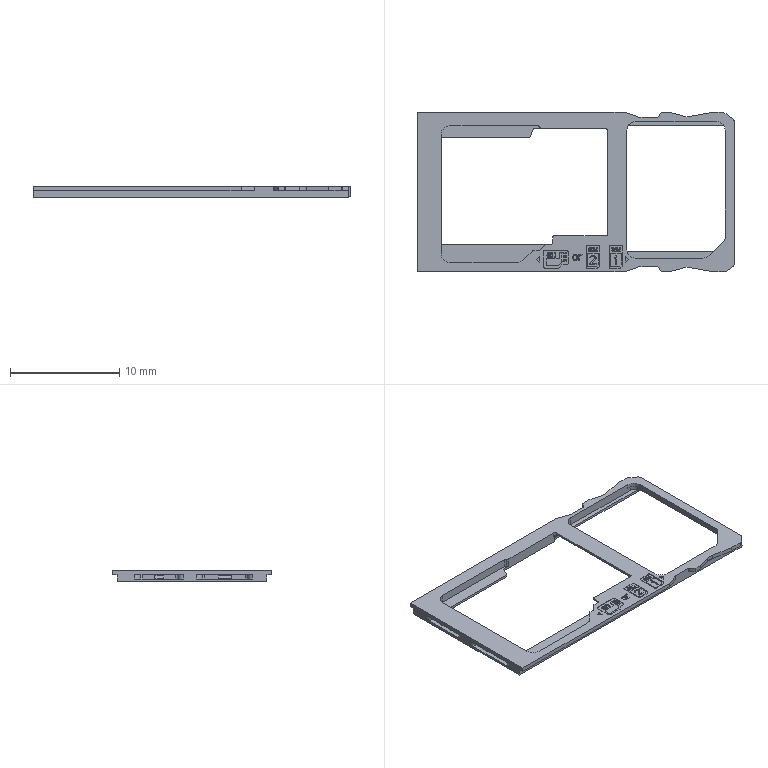Part | Creo | 1 solid | 549 faces | box 29.01 x 14.6 x 1 mm | volume 102.876 mm3 | plane 443 | cylinder 99 | other 7 | commonest cylinder face diameters 0.2 x34 0.3 x19 0.4 x14 0.24 x8 1 x7 1.6 x7